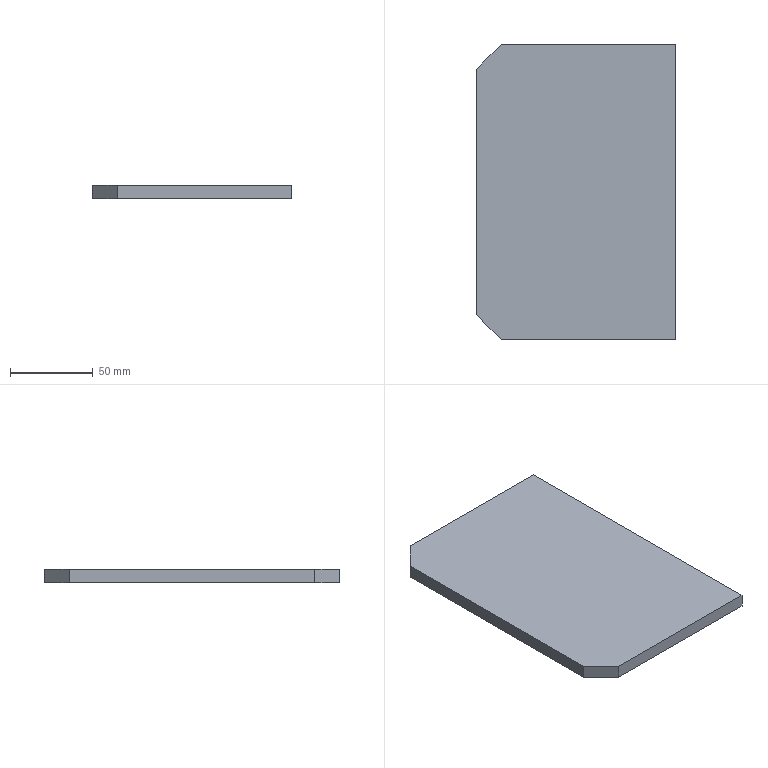Part | STEP file | 04-Rib plate 1 | 1 solid | 8 faces | box 120 x 178 x 8 mm | volume 169080 mm3 | plane 8
STEP:
#1=CARTESIAN_POINT('',(0.,0.,0.));
#2=DIRECTION('',(0.,0.,1.));
#3=DIRECTION('',(1.,0.,0.));
#4=AXIS2_PLACEMENT_3D('',#1,#2,#3);
#5=CARTESIAN_POINT('',(0.,-178.,0.));
#6=VERTEX_POINT('',#5);
#7=CARTESIAN_POINT('',(0.,0.,0.));
#8=VERTEX_POINT('',#7);
#9=CARTESIAN_POINT('',(0.,0.,0.));
#10=DIRECTION('',(0.,1.,0.));
#11=VECTOR('',#10,1.);
#12=LINE('',#9,#11);
#13=CARTESIAN_POINT('',(0.,0.,8.));
#14=DIRECTION('',(-1.,0.,0.));
#15=DIRECTION('',(0.,-1.,0.));
#16=AXIS2_PLACEMENT_3D('',#13,#14,#15);
#17=PLANE('',#16);
#18=CARTESIAN_POINT('',(0.,-8.));
#19=DIRECTION('',(-1.,0.));
#20=VECTOR('',#19,1.);
#21=LINE('',#18,#20);
#22=(GEOMETRIC_REPRESENTATION_CONTEXT(2)PARAMETRIC_REPRESENTATION_CONTEXT()REPRESENTATION_CONTEXT('',''));
#23=DEFINITIONAL_REPRESENTATION('',(#21),#22);
#24=PCURVE('',#17,#23);
#25=CARTESIAN_POINT('',(0.,0.,0.));
#26=DIRECTION('',(0.,0.,-1.));
#27=DIRECTION('',(-1.,0.,0.));
#28=AXIS2_PLACEMENT_3D('',#25,#26,#27);
#29=PLANE('',#28);
#30=CARTESIAN_POINT('',(0.,0.));
#31=DIRECTION('',(0.,1.));
#32=VECTOR('',#31,1.);
#33=LINE('',#30,#32);
#34=(GEOMETRIC_REPRESENTATION_CONTEXT(2)PARAMETRIC_REPRESENTATION_CONTEXT()REPRESENTATION_CONTEXT('',''));
#35=DEFINITIONAL_REPRESENTATION('',(#33),#34);
#36=PCURVE('',#29,#35);
#37=SURFACE_CURVE('',#12,(#24,#36),.PCURVE_S1.);
#38=EDGE_CURVE('',#6,#8,#37,.T.);
#39=ORIENTED_EDGE('',*,*,#38,.T.);
#40=CARTESIAN_POINT('',(0.,0.,8.));
#41=VERTEX_POINT('',#40);
#42=CARTESIAN_POINT('',(0.,0.,8.));
#43=DIRECTION('',(0.,0.,-1.));
#44=VECTOR('',#43,1.);
#45=LINE('',#42,#44);
#46=CARTESIAN_POINT('',(0.,0.));
#47=DIRECTION('',(0.,-1.));
#48=VECTOR('',#47,1.);
#49=LINE('',#46,#48);
#50=(GEOMETRIC_REPRESENTATION_CONTEXT(2)PARAMETRIC_REPRESENTATION_CONTEXT()REPRESENTATION_CONTEXT('',''));
#51=DEFINITIONAL_REPRESENTATION('',(#49),#50);
#52=PCURVE('',#17,#51);
#53=CARTESIAN_POINT('',(0.,0.,8.));
#54=DIRECTION('',(0.,-1.,0.));
#55=DIRECTION('',(1.,0.,0.));
#56=AXIS2_PLACEMENT_3D('',#53,#54,#55);
#57=PLANE('',#56);
#58=CARTESIAN_POINT('',(0.,0.));
#59=DIRECTION('',(0.,-1.));
#60=VECTOR('',#59,1.);
#61=LINE('',#58,#60);
#62=(GEOMETRIC_REPRESENTATION_CONTEXT(2)PARAMETRIC_REPRESENTATION_CONTEXT()REPRESENTATION_CONTEXT('',''));
#63=DEFINITIONAL_REPRESENTATION('',(#61),#62);
#64=PCURVE('',#57,#63);
#65=SURFACE_CURVE('',#45,(#52,#64),.PCURVE_S1.);
#66=EDGE_CURVE('',#41,#8,#65,.T.);
#67=ORIENTED_EDGE('',*,*,#66,.F.);
#68=CARTESIAN_POINT('',(0.,-178.,8.));
#69=VERTEX_POINT('',#68);
#70=CARTESIAN_POINT('',(0.,0.,8.));
#71=DIRECTION('',(0.,1.,0.));
#72=VECTOR('',#71,1.);
#73=LINE('',#70,#72);
#74=CARTESIAN_POINT('',(0.,0.));
#75=DIRECTION('',(-1.,0.));
#76=VECTOR('',#75,1.);
#77=LINE('',#74,#76);
#78=(GEOMETRIC_REPRESENTATION_CONTEXT(2)PARAMETRIC_REPRESENTATION_CONTEXT()REPRESENTATION_CONTEXT('',''));
#79=DEFINITIONAL_REPRESENTATION('',(#77),#78);
#80=PCURVE('',#17,#79);
#81=CARTESIAN_POINT('',(0.,0.,8.));
#82=DIRECTION('',(0.,0.,-1.));
#83=DIRECTION('',(-1.,0.,0.));
#84=AXIS2_PLACEMENT_3D('',#81,#82,#83);
#85=PLANE('',#84);
#86=CARTESIAN_POINT('',(0.,0.));
#87=DIRECTION('',(0.,1.));
#88=VECTOR('',#87,1.);
#89=LINE('',#86,#88);
#90=(GEOMETRIC_REPRESENTATION_CONTEXT(2)PARAMETRIC_REPRESENTATION_CONTEXT()REPRESENTATION_CONTEXT('',''));
#91=DEFINITIONAL_REPRESENTATION('',(#89),#90);
#92=PCURVE('',#85,#91);
#93=SURFACE_CURVE('',#73,(#80,#92),.PCURVE_S1.);
#94=EDGE_CURVE('',#69,#41,#93,.T.);
#95=ORIENTED_EDGE('',*,*,#94,.F.);
#96=CARTESIAN_POINT('',(0.,-178.,8.));
#97=DIRECTION('',(0.,0.,-1.));
#98=VECTOR('',#97,1.);
#99=LINE('',#96,#98);
#100=CARTESIAN_POINT('',(178.,0.));
#101=DIRECTION('',(0.,-1.));
#102=VECTOR('',#101,1.);
#103=LINE('',#100,#102);
#104=(GEOMETRIC_REPRESENTATION_CONTEXT(2)PARAMETRIC_REPRESENTATION_CONTEXT()REPRESENTATION_CONTEXT('',''));
#105=DEFINITIONAL_REPRESENTATION('',(#103),#104);
#106=PCURVE('',#17,#105);
#107=CARTESIAN_POINT('',(0.,-178.,8.));
#108=DIRECTION('',(0.,1.,0.));
#109=DIRECTION('',(-1.,0.,0.));
#110=AXIS2_PLACEMENT_3D('',#107,#108,#109);
#111=PLANE('',#110);
#112=CARTESIAN_POINT('',(0.,0.));
#113=DIRECTION('',(0.,-1.));
#114=VECTOR('',#113,1.);
#115=LINE('',#112,#114);
#116=(GEOMETRIC_REPRESENTATION_CONTEXT(2)PARAMETRIC_REPRESENTATION_CONTEXT()REPRESENTATION_CONTEXT('',''));
#117=DEFINITIONAL_REPRESENTATION('',(#115),#116);
#118=PCURVE('',#111,#117);
#119=SURFACE_CURVE('',#99,(#106,#118),.PCURVE_S1.);
#120=EDGE_CURVE('',#69,#6,#119,.T.);
#121=ORIENTED_EDGE('',*,*,#120,.T.);
#122=EDGE_LOOP('',(#39,#67,#95,#121));
#123=FACE_BOUND('',#122,.T.);
#124=ADVANCED_FACE('',(#123),#17,.F.);
#125=CARTESIAN_POINT('',(-105.,0.,0.));
#126=VERTEX_POINT('',#125);
#127=CARTESIAN_POINT('',(0.,0.,0.));
#128=DIRECTION('',(-1.,0.,0.));
#129=VECTOR('',#128,1.);
#130=LINE('',#127,#129);
#131=CARTESIAN_POINT('',(0.,-8.));
#132=DIRECTION('',(-1.,0.));
#133=VECTOR('',#132,1.);
#134=LINE('',#131,#133);
#135=(GEOMETRIC_REPRESENTATION_CONTEXT(2)PARAMETRIC_REPRESENTATION_CONTEXT()REPRESENTATION_CONTEXT('',''));
#136=DEFINITIONAL_REPRESENTATION('',(#134),#135);
#137=PCURVE('',#57,#136);
#138=CARTESIAN_POINT('',(0.,0.));
#139=DIRECTION('',(1.,0.));
#140=VECTOR('',#139,1.);
#141=LINE('',#138,#140);
#142=(GEOMETRIC_REPRESENTATION_CONTEXT(2)PARAMETRIC_REPRESENTATION_CONTEXT()REPRESENTATION_CONTEXT('',''));
#143=DEFINITIONAL_REPRESENTATION('',(#141),#142);
#144=PCURVE('',#29,#143);
#145=SURFACE_CURVE('',#130,(#137,#144),.PCURVE_S1.);
#146=EDGE_CURVE('',#8,#126,#145,.T.);
#147=ORIENTED_EDGE('',*,*,#146,.T.);
#148=CARTESIAN_POINT('',(-105.,0.,8.));
#149=VERTEX_POINT('',#148);
#150=CARTESIAN_POINT('',(-105.,0.,8.));
#151=DIRECTION('',(0.,0.,-1.));
#152=VECTOR('',#151,1.);
#153=LINE('',#150,#152);
#154=CARTESIAN_POINT('',(-105.,0.));
#155=DIRECTION('',(0.,-1.));
#156=VECTOR('',#155,1.);
#157=LINE('',#154,#156);
#158=(GEOMETRIC_REPRESENTATION_CONTEXT(2)PARAMETRIC_REPRESENTATION_CONTEXT()REPRESENTATION_CONTEXT('',''));
#159=DEFINITIONAL_REPRESENTATION('',(#157),#158);
#160=PCURVE('',#57,#159);
#161=CARTESIAN_POINT('',(-105.,0.,8.));
#162=DIRECTION('',(0.7071,-0.7071,0.));
#163=DIRECTION('',(0.7071,0.7071,0.));
#164=AXIS2_PLACEMENT_3D('',#161,#162,#163);
#165=PLANE('',#164);
#166=CARTESIAN_POINT('',(0.,0.));
#167=DIRECTION('',(0.,-1.));
#168=VECTOR('',#167,1.);
#169=LINE('',#166,#168);
#170=(GEOMETRIC_REPRESENTATION_CONTEXT(2)PARAMETRIC_REPRESENTATION_CONTEXT()REPRESENTATION_CONTEXT('',''));
#171=DEFINITIONAL_REPRESENTATION('',(#169),#170);
#172=PCURVE('',#165,#171);
#173=SURFACE_CURVE('',#153,(#160,#172),.PCURVE_S1.);
#174=EDGE_CURVE('',#149,#126,#173,.T.);
#175=ORIENTED_EDGE('',*,*,#174,.F.);
#176=CARTESIAN_POINT('',(0.,0.,8.));
#177=DIRECTION('',(-1.,0.,0.));
#178=VECTOR('',#177,1.);
#179=LINE('',#176,#178);
#180=CARTESIAN_POINT('',(0.,0.));
#181=DIRECTION('',(-1.,0.));
#182=VECTOR('',#181,1.);
#183=LINE('',#180,#182);
#184=(GEOMETRIC_REPRESENTATION_CONTEXT(2)PARAMETRIC_REPRESENTATION_CONTEXT()REPRESENTATION_CONTEXT('',''));
#185=DEFINITIONAL_REPRESENTATION('',(#183),#184);
#186=PCURVE('',#57,#185);
#187=CARTESIAN_POINT('',(0.,0.));
#188=DIRECTION('',(1.,0.));
#189=VECTOR('',#188,1.);
#190=LINE('',#187,#189);
#191=(GEOMETRIC_REPRESENTATION_CONTEXT(2)PARAMETRIC_REPRESENTATION_CONTEXT()REPRESENTATION_CONTEXT('',''));
#192=DEFINITIONAL_REPRESENTATION('',(#190),#191);
#193=PCURVE('',#85,#192);
#194=SURFACE_CURVE('',#179,(#186,#193),.PCURVE_S1.);
#195=EDGE_CURVE('',#41,#149,#194,.T.);
#196=ORIENTED_EDGE('',*,*,#195,.F.);
#197=ORIENTED_EDGE('',*,*,#66,.T.);
#198=EDGE_LOOP('',(#147,#175,#196,#197));
#199=FACE_BOUND('',#198,.T.);
#200=ADVANCED_FACE('',(#199),#57,.F.);
#201=CARTESIAN_POINT('',(-120.,-15.,0.));
#202=VERTEX_POINT('',#201);
#203=CARTESIAN_POINT('',(-105.,0.,0.));
#204=DIRECTION('',(-0.7071,-0.7071,0.));
#205=VECTOR('',#204,1.);
#206=LINE('',#203,#205);
#207=CARTESIAN_POINT('',(0.,-8.));
#208=DIRECTION('',(-1.,0.));
#209=VECTOR('',#208,1.);
#210=LINE('',#207,#209);
#211=(GEOMETRIC_REPRESENTATION_CONTEXT(2)PARAMETRIC_REPRESENTATION_CONTEXT()REPRESENTATION_CONTEXT('',''));
#212=DEFINITIONAL_REPRESENTATION('',(#210),#211);
#213=PCURVE('',#165,#212);
#214=CARTESIAN_POINT('',(105.,0.));
#215=DIRECTION('',(0.7071,-0.7071));
#216=VECTOR('',#215,1.);
#217=LINE('',#214,#216);
#218=(GEOMETRIC_REPRESENTATION_CONTEXT(2)PARAMETRIC_REPRESENTATION_CONTEXT()REPRESENTATION_CONTEXT('',''));
#219=DEFINITIONAL_REPRESENTATION('',(#217),#218);
#220=PCURVE('',#29,#219);
#221=SURFACE_CURVE('',#206,(#213,#220),.PCURVE_S1.);
#222=EDGE_CURVE('',#126,#202,#221,.T.);
#223=ORIENTED_EDGE('',*,*,#222,.T.);
#224=CARTESIAN_POINT('',(-120.,-15.,8.));
#225=VERTEX_POINT('',#224);
#226=CARTESIAN_POINT('',(-120.,-15.,8.));
#227=DIRECTION('',(0.,0.,-1.));
#228=VECTOR('',#227,1.);
#229=LINE('',#226,#228);
#230=CARTESIAN_POINT('',(-21.213,0.));
#231=DIRECTION('',(0.,-1.));
#232=VECTOR('',#231,1.);
#233=LINE('',#230,#232);
#234=(GEOMETRIC_REPRESENTATION_CONTEXT(2)PARAMETRIC_REPRESENTATION_CONTEXT()REPRESENTATION_CONTEXT('',''));
#235=DEFINITIONAL_REPRESENTATION('',(#233),#234);
#236=PCURVE('',#165,#235);
#237=CARTESIAN_POINT('',(-120.,-15.,8.));
#238=DIRECTION('',(1.,0.,0.));
#239=DIRECTION('',(0.,1.,0.));
#240=AXIS2_PLACEMENT_3D('',#237,#238,#239);
#241=PLANE('',#240);
#242=CARTESIAN_POINT('',(0.,0.));
#243=DIRECTION('',(0.,-1.));
#244=VECTOR('',#243,1.);
#245=LINE('',#242,#244);
#246=(GEOMETRIC_REPRESENTATION_CONTEXT(2)PARAMETRIC_REPRESENTATION_CONTEXT()REPRESENTATION_CONTEXT('',''));
#247=DEFINITIONAL_REPRESENTATION('',(#245),#246);
#248=PCURVE('',#241,#247);
#249=SURFACE_CURVE('',#229,(#236,#248),.PCURVE_S1.);
#250=EDGE_CURVE('',#225,#202,#249,.T.);
#251=ORIENTED_EDGE('',*,*,#250,.F.);
#252=CARTESIAN_POINT('',(-105.,0.,8.));
#253=DIRECTION('',(-0.7071,-0.7071,0.));
#254=VECTOR('',#253,1.);
#255=LINE('',#252,#254);
#256=CARTESIAN_POINT('',(0.,0.));
#257=DIRECTION('',(-1.,0.));
#258=VECTOR('',#257,1.);
#259=LINE('',#256,#258);
#260=(GEOMETRIC_REPRESENTATION_CONTEXT(2)PARAMETRIC_REPRESENTATION_CONTEXT()REPRESENTATION_CONTEXT('',''));
#261=DEFINITIONAL_REPRESENTATION('',(#259),#260);
#262=PCURVE('',#165,#261);
#263=CARTESIAN_POINT('',(105.,0.));
#264=DIRECTION('',(0.7071,-0.7071));
#265=VECTOR('',#264,1.);
#266=LINE('',#263,#265);
#267=(GEOMETRIC_REPRESENTATION_CONTEXT(2)PARAMETRIC_REPRESENTATION_CONTEXT()REPRESENTATION_CONTEXT('',''));
#268=DEFINITIONAL_REPRESENTATION('',(#266),#267);
#269=PCURVE('',#85,#268);
#270=SURFACE_CURVE('',#255,(#262,#269),.PCURVE_S1.);
#271=EDGE_CURVE('',#149,#225,#270,.T.);
#272=ORIENTED_EDGE('',*,*,#271,.F.);
#273=ORIENTED_EDGE('',*,*,#174,.T.);
#274=EDGE_LOOP('',(#223,#251,#272,#273));
#275=FACE_BOUND('',#274,.T.);
#276=ADVANCED_FACE('',(#275),#165,.F.);
#277=CARTESIAN_POINT('',(-120.,-163.,0.));
#278=VERTEX_POINT('',#277);
#279=CARTESIAN_POINT('',(-120.,-15.,0.));
#280=DIRECTION('',(0.,-1.,0.));
#281=VECTOR('',#280,1.);
#282=LINE('',#279,#281);
#283=CARTESIAN_POINT('',(0.,-8.));
#284=DIRECTION('',(-1.,0.));
#285=VECTOR('',#284,1.);
#286=LINE('',#283,#285);
#287=(GEOMETRIC_REPRESENTATION_CONTEXT(2)PARAMETRIC_REPRESENTATION_CONTEXT()REPRESENTATION_CONTEXT('',''));
#288=DEFINITIONAL_REPRESENTATION('',(#286),#287);
#289=PCURVE('',#241,#288);
#290=CARTESIAN_POINT('',(120.,-15.));
#291=DIRECTION('',(0.,-1.));
#292=VECTOR('',#291,1.);
#293=LINE('',#290,#292);
#294=(GEOMETRIC_REPRESENTATION_CONTEXT(2)PARAMETRIC_REPRESENTATION_CONTEXT()REPRESENTATION_CONTEXT('',''));
#295=DEFINITIONAL_REPRESENTATION('',(#293),#294);
#296=PCURVE('',#29,#295);
#297=SURFACE_CURVE('',#282,(#289,#296),.PCURVE_S1.);
#298=EDGE_CURVE('',#202,#278,#297,.T.);
#299=ORIENTED_EDGE('',*,*,#298,.T.);
#300=CARTESIAN_POINT('',(-120.,-163.,8.));
#301=VERTEX_POINT('',#300);
#302=CARTESIAN_POINT('',(-120.,-163.,8.));
#303=DIRECTION('',(0.,0.,-1.));
#304=VECTOR('',#303,1.);
#305=LINE('',#302,#304);
#306=CARTESIAN_POINT('',(-148.,0.));
#307=DIRECTION('',(0.,-1.));
#308=VECTOR('',#307,1.);
#309=LINE('',#306,#308);
#310=(GEOMETRIC_REPRESENTATION_CONTEXT(2)PARAMETRIC_REPRESENTATION_CONTEXT()REPRESENTATION_CONTEXT('',''));
#311=DEFINITIONAL_REPRESENTATION('',(#309),#310);
#312=PCURVE('',#241,#311);
#313=CARTESIAN_POINT('',(-120.,-163.,8.));
#314=DIRECTION('',(0.7071,0.7071,0.));
#315=DIRECTION('',(-0.7071,0.7071,0.));
#316=AXIS2_PLACEMENT_3D('',#313,#314,#315);
#317=PLANE('',#316);
#318=CARTESIAN_POINT('',(0.,0.));
#319=DIRECTION('',(0.,-1.));
#320=VECTOR('',#319,1.);
#321=LINE('',#318,#320);
#322=(GEOMETRIC_REPRESENTATION_CONTEXT(2)PARAMETRIC_REPRESENTATION_CONTEXT()REPRESENTATION_CONTEXT('',''));
#323=DEFINITIONAL_REPRESENTATION('',(#321),#322);
#324=PCURVE('',#317,#323);
#325=SURFACE_CURVE('',#305,(#312,#324),.PCURVE_S1.);
#326=EDGE_CURVE('',#301,#278,#325,.T.);
#327=ORIENTED_EDGE('',*,*,#326,.F.);
#328=CARTESIAN_POINT('',(-120.,-15.,8.));
#329=DIRECTION('',(0.,-1.,0.));
#330=VECTOR('',#329,1.);
#331=LINE('',#328,#330);
#332=CARTESIAN_POINT('',(0.,0.));
#333=DIRECTION('',(-1.,0.));
#334=VECTOR('',#333,1.);
#335=LINE('',#332,#334);
#336=(GEOMETRIC_REPRESENTATION_CONTEXT(2)PARAMETRIC_REPRESENTATION_CONTEXT()REPRESENTATION_CONTEXT('',''));
#337=DEFINITIONAL_REPRESENTATION('',(#335),#336);
#338=PCURVE('',#241,#337);
#339=CARTESIAN_POINT('',(120.,-15.));
#340=DIRECTION('',(0.,-1.));
#341=VECTOR('',#340,1.);
#342=LINE('',#339,#341);
#343=(GEOMETRIC_REPRESENTATION_CONTEXT(2)PARAMETRIC_REPRESENTATION_CONTEXT()REPRESENTATION_CONTEXT('',''));
#344=DEFINITIONAL_REPRESENTATION('',(#342),#343);
#345=PCURVE('',#85,#344);
#346=SURFACE_CURVE('',#331,(#338,#345),.PCURVE_S1.);
#347=EDGE_CURVE('',#225,#301,#346,.T.);
#348=ORIENTED_EDGE('',*,*,#347,.F.);
#349=ORIENTED_EDGE('',*,*,#250,.T.);
#350=EDGE_LOOP('',(#299,#327,#348,#349));
#351=FACE_BOUND('',#350,.T.);
#352=ADVANCED_FACE('',(#351),#241,.F.);
#353=CARTESIAN_POINT('',(-105.,-178.,0.));
#354=VERTEX_POINT('',#353);
#355=CARTESIAN_POINT('',(-120.,-163.,0.));
#356=DIRECTION('',(0.7071,-0.7071,0.));
#357=VECTOR('',#356,1.);
#358=LINE('',#355,#357);
#359=CARTESIAN_POINT('',(0.,-8.));
#360=DIRECTION('',(-1.,0.));
#361=VECTOR('',#360,1.);
#362=LINE('',#359,#361);
#363=(GEOMETRIC_REPRESENTATION_CONTEXT(2)PARAMETRIC_REPRESENTATION_CONTEXT()REPRESENTATION_CONTEXT('',''));
#364=DEFINITIONAL_REPRESENTATION('',(#362),#363);
#365=PCURVE('',#317,#364);
#366=CARTESIAN_POINT('',(120.,-163.));
#367=DIRECTION('',(-0.7071,-0.7071));
#368=VECTOR('',#367,1.);
#369=LINE('',#366,#368);
#370=(GEOMETRIC_REPRESENTATION_CONTEXT(2)PARAMETRIC_REPRESENTATION_CONTEXT()REPRESENTATION_CONTEXT('',''));
#371=DEFINITIONAL_REPRESENTATION('',(#369),#370);
#372=PCURVE('',#29,#371);
#373=SURFACE_CURVE('',#358,(#365,#372),.PCURVE_S1.);
#374=EDGE_CURVE('',#278,#354,#373,.T.);
#375=ORIENTED_EDGE('',*,*,#374,.T.);
#376=CARTESIAN_POINT('',(-105.,-178.,8.));
#377=VERTEX_POINT('',#376);
#378=CARTESIAN_POINT('',(-105.,-178.,8.));
#379=DIRECTION('',(0.,0.,-1.));
#380=VECTOR('',#379,1.);
#381=LINE('',#378,#380);
#382=CARTESIAN_POINT('',(-21.213,0.));
#383=DIRECTION('',(0.,-1.));
#384=VECTOR('',#383,1.);
#385=LINE('',#382,#384);
#386=(GEOMETRIC_REPRESENTATION_CONTEXT(2)PARAMETRIC_REPRESENTATION_CONTEXT()REPRESENTATION_CONTEXT('',''));
#387=DEFINITIONAL_REPRESENTATION('',(#385),#386);
#388=PCURVE('',#317,#387);
#389=CARTESIAN_POINT('',(105.,0.));
#390=DIRECTION('',(0.,-1.));
#391=VECTOR('',#390,1.);
#392=LINE('',#389,#391);
#393=(GEOMETRIC_REPRESENTATION_CONTEXT(2)PARAMETRIC_REPRESENTATION_CONTEXT()REPRESENTATION_CONTEXT('',''));
#394=DEFINITIONAL_REPRESENTATION('',(#392),#393);
#395=PCURVE('',#111,#394);
#396=SURFACE_CURVE('',#381,(#388,#395),.PCURVE_S1.);
#397=EDGE_CURVE('',#377,#354,#396,.T.);
#398=ORIENTED_EDGE('',*,*,#397,.F.);
#399=CARTESIAN_POINT('',(-120.,-163.,8.));
#400=DIRECTION('',(0.7071,-0.7071,0.));
#401=VECTOR('',#400,1.);
#402=LINE('',#399,#401);
#403=CARTESIAN_POINT('',(0.,0.));
#404=DIRECTION('',(-1.,0.));
#405=VECTOR('',#404,1.);
#406=LINE('',#403,#405);
#407=(GEOMETRIC_REPRESENTATION_CONTEXT(2)PARAMETRIC_REPRESENTATION_CONTEXT()REPRESENTATION_CONTEXT('',''));
#408=DEFINITIONAL_REPRESENTATION('',(#406),#407);
#409=PCURVE('',#317,#408);
#410=CARTESIAN_POINT('',(120.,-163.));
#411=DIRECTION('',(-0.7071,-0.7071));
#412=VECTOR('',#411,1.);
#413=LINE('',#410,#412);
#414=(GEOMETRIC_REPRESENTATION_CONTEXT(2)PARAMETRIC_REPRESENTATION_CONTEXT()REPRESENTATION_CONTEXT('',''));
#415=DEFINITIONAL_REPRESENTATION('',(#413),#414);
#416=PCURVE('',#85,#415);
#417=SURFACE_CURVE('',#402,(#409,#416),.PCURVE_S1.);
#418=EDGE_CURVE('',#301,#377,#417,.T.);
#419=ORIENTED_EDGE('',*,*,#418,.F.);
#420=ORIENTED_EDGE('',*,*,#326,.T.);
#421=EDGE_LOOP('',(#375,#398,#419,#420));
#422=FACE_BOUND('',#421,.T.);
#423=ADVANCED_FACE('',(#422),#317,.F.);
#424=CARTESIAN_POINT('',(0.,-178.,0.));
#425=DIRECTION('',(1.,0.,0.));
#426=VECTOR('',#425,1.);
#427=LINE('',#424,#426);
#428=CARTESIAN_POINT('',(0.,-8.));
#429=DIRECTION('',(-1.,0.));
#430=VECTOR('',#429,1.);
#431=LINE('',#428,#430);
#432=(GEOMETRIC_REPRESENTATION_CONTEXT(2)PARAMETRIC_REPRESENTATION_CONTEXT()REPRESENTATION_CONTEXT('',''));
#433=DEFINITIONAL_REPRESENTATION('',(#431),#432);
#434=PCURVE('',#111,#433);
#435=CARTESIAN_POINT('',(0.,-178.));
#436=DIRECTION('',(-1.,0.));
#437=VECTOR('',#436,1.);
#438=LINE('',#435,#437);
#439=(GEOMETRIC_REPRESENTATION_CONTEXT(2)PARAMETRIC_REPRESENTATION_CONTEXT()REPRESENTATION_CONTEXT('',''));
#440=DEFINITIONAL_REPRESENTATION('',(#438),#439);
#441=PCURVE('',#29,#440);
#442=SURFACE_CURVE('',#427,(#434,#441),.PCURVE_S1.);
#443=EDGE_CURVE('',#354,#6,#442,.T.);
#444=ORIENTED_EDGE('',*,*,#443,.T.);
#445=ORIENTED_EDGE('',*,*,#120,.F.);
#446=CARTESIAN_POINT('',(0.,-178.,8.));
#447=DIRECTION('',(1.,0.,0.));
#448=VECTOR('',#447,1.);
#449=LINE('',#446,#448);
#450=CARTESIAN_POINT('',(0.,0.));
#451=DIRECTION('',(-1.,0.));
#452=VECTOR('',#451,1.);
#453=LINE('',#450,#452);
#454=(GEOMETRIC_REPRESENTATION_CONTEXT(2)PARAMETRIC_REPRESENTATION_CONTEXT()REPRESENTATION_CONTEXT('',''));
#455=DEFINITIONAL_REPRESENTATION('',(#453),#454);
#456=PCURVE('',#111,#455);
#457=CARTESIAN_POINT('',(0.,-178.));
#458=DIRECTION('',(-1.,0.));
#459=VECTOR('',#458,1.);
#460=LINE('',#457,#459);
#461=(GEOMETRIC_REPRESENTATION_CONTEXT(2)PARAMETRIC_REPRESENTATION_CONTEXT()REPRESENTATION_CONTEXT('',''));
#462=DEFINITIONAL_REPRESENTATION('',(#460),#461);
#463=PCURVE('',#85,#462);
#464=SURFACE_CURVE('',#449,(#456,#463),.PCURVE_S1.);
#465=EDGE_CURVE('',#377,#69,#464,.T.);
#466=ORIENTED_EDGE('',*,*,#465,.F.);
#467=ORIENTED_EDGE('',*,*,#397,.T.);
#468=EDGE_LOOP('',(#444,#445,#466,#467));
#469=FACE_BOUND('',#468,.T.);
#470=ADVANCED_FACE('',(#469),#111,.F.);
#471=ORIENTED_EDGE('',*,*,#94,.T.);
#472=ORIENTED_EDGE('',*,*,#195,.T.);
#473=ORIENTED_EDGE('',*,*,#271,.T.);
#474=ORIENTED_EDGE('',*,*,#347,.T.);
#475=ORIENTED_EDGE('',*,*,#418,.T.);
#476=ORIENTED_EDGE('',*,*,#465,.T.);
#477=EDGE_LOOP('',(#471,#472,#473,#474,#475,#476));
#478=FACE_BOUND('',#477,.T.);
#479=ADVANCED_FACE('',(#478),#85,.F.);
#480=ORIENTED_EDGE('',*,*,#38,.F.);
#481=ORIENTED_EDGE('',*,*,#443,.F.);
#482=ORIENTED_EDGE('',*,*,#374,.F.);
#483=ORIENTED_EDGE('',*,*,#298,.F.);
#484=ORIENTED_EDGE('',*,*,#222,.F.);
#485=ORIENTED_EDGE('',*,*,#146,.F.);
#486=EDGE_LOOP('',(#480,#481,#482,#483,#484,#485));
#487=FACE_BOUND('',#486,.T.);
#488=ADVANCED_FACE('',(#487),#29,.T.);
#489=CLOSED_SHELL('',(#124,#200,#276,#352,#423,#470,#479,#488));
#490=MANIFOLD_SOLID_BREP('',#489);
#491=(LENGTH_UNIT()NAMED_UNIT(*)SI_UNIT(.MILLI.,.METRE.));
#492=UNCERTAINTY_MEASURE_WITH_UNIT(LENGTH_MEASURE(0.0000001),#491,'','');
#493=(NAMED_UNIT(*)PLANE_ANGLE_UNIT()SI_UNIT($,.RADIAN.));
#494=(NAMED_UNIT(*)SI_UNIT($,.STERADIAN.)SOLID_ANGLE_UNIT());
#495=(GEOMETRIC_REPRESENTATION_CONTEXT(3)GLOBAL_UNCERTAINTY_ASSIGNED_CONTEXT((#492))GLOBAL_UNIT_ASSIGNED_CONTEXT((#491,#493,#494))REPRESENTATION_CONTEXT('',''));
#496=ADVANCED_BREP_SHAPE_REPRESENTATION('',(#4,#490),#495);